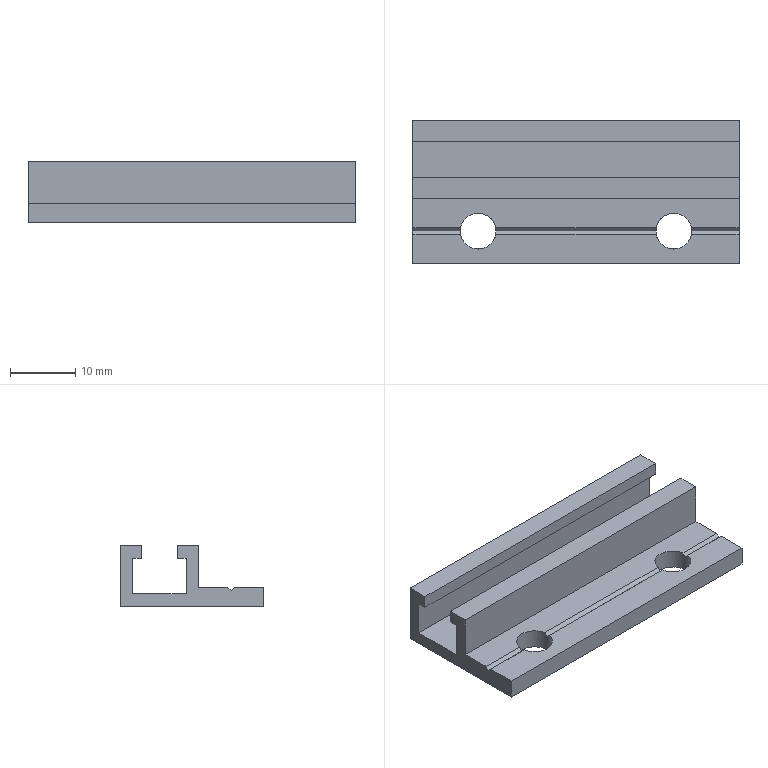Part | STEP file | SENCF5-50 | 1 solid | 27 faces | box 50 x 22 x 9.5 mm | volume 4243 mm3 | plane 23 | cylinder 4 | commonest cylinder face diameters 5.5 x4
STEP:
#1=CARTESIAN_POINT('',(42.704,-0.5,3.));
#2=VERTEX_POINT('',#1);
#3=CARTESIAN_POINT('',(42.75,0.,2.5));
#4=VERTEX_POINT('',#3);
#5=CARTESIAN_POINT('',(42.704,-0.5,3.));
#6=CARTESIAN_POINT('',(42.735,-0.335,2.835));
#7=CARTESIAN_POINT('',(42.75,-0.1678,2.668));
#8=CARTESIAN_POINT('',(42.75,0.,2.5));
#9=(BOUNDED_CURVE()B_SPLINE_CURVE(3,(#5,#6,#7,#8),.UNSPECIFIED.,.F.,.F.)B_SPLINE_CURVE_WITH_KNOTS((4,4),(4.53,4.712),.UNSPECIFIED.)CURVE()GEOMETRIC_REPRESENTATION_ITEM()RATIONAL_B_SPLINE_CURVE((1.,0.9972,0.9972,1.))REPRESENTATION_ITEM(''));
#10=EDGE_CURVE('',#2,#4,#9,.T.);
#11=ORIENTED_EDGE('',*,*,#10,.T.);
#12=CARTESIAN_POINT('',(42.75,0.,0.));
#13=VERTEX_POINT('',#12);
#14=CARTESIAN_POINT('',(42.75,0.,9.5));
#15=DIRECTION('',(0.,0.,-1.));
#16=VECTOR('',#15,1000.);
#17=LINE('',#14,#16);
#18=EDGE_CURVE('',#4,#13,#17,.T.);
#19=ORIENTED_EDGE('',*,*,#18,.T.);
#20=CARTESIAN_POINT('',(37.25,0.,0.));
#21=VERTEX_POINT('',#20);
#22=CARTESIAN_POINT('',(40.,0.,0.));
#23=DIRECTION('',(0.,0.,1.));
#24=DIRECTION('',(1.,0.,0.));
#25=AXIS2_PLACEMENT_3D('',#22,#23,#24);
#26=CIRCLE('',#25,2.75);
#27=EDGE_CURVE('',#21,#13,#26,.T.);
#28=ORIENTED_EDGE('',*,*,#27,.F.);
#29=CARTESIAN_POINT('',(37.25,0.,2.5));
#30=VERTEX_POINT('',#29);
#31=CARTESIAN_POINT('',(37.25,0.,9.5));
#32=DIRECTION('',(0.,0.,-1.));
#33=VECTOR('',#32,1000.);
#34=LINE('',#31,#33);
#35=EDGE_CURVE('',#30,#21,#34,.T.);
#36=ORIENTED_EDGE('',*,*,#35,.F.);
#37=CARTESIAN_POINT('',(37.296,-0.5,3.));
#38=VERTEX_POINT('',#37);
#39=CARTESIAN_POINT('',(37.25,0.,2.5));
#40=CARTESIAN_POINT('',(37.25,-0.1678,2.668));
#41=CARTESIAN_POINT('',(37.265,-0.335,2.835));
#42=CARTESIAN_POINT('',(37.296,-0.5,3.));
#43=(BOUNDED_CURVE()B_SPLINE_CURVE(3,(#39,#40,#41,#42),.UNSPECIFIED.,.F.,.F.)B_SPLINE_CURVE_WITH_KNOTS((4,4),(1.571,1.754),.UNSPECIFIED.)CURVE()GEOMETRIC_REPRESENTATION_ITEM()RATIONAL_B_SPLINE_CURVE((1.,0.9972,0.9972,1.))REPRESENTATION_ITEM(''));
#44=EDGE_CURVE('',#30,#38,#43,.T.);
#45=ORIENTED_EDGE('',*,*,#44,.T.);
#46=CARTESIAN_POINT('',(40.,0.,3.));
#47=DIRECTION('',(0.,0.,1.));
#48=DIRECTION('',(0.,1.,0.));
#49=AXIS2_PLACEMENT_3D('',#46,#47,#48);
#50=CIRCLE('',#49,2.75);
#51=EDGE_CURVE('',#38,#2,#50,.T.);
#52=ORIENTED_EDGE('',*,*,#51,.T.);
#53=EDGE_LOOP('',(#11,#19,#28,#36,#45,#52));
#54=FACE_OUTER_BOUND('',#53,.T.);
#55=CARTESIAN_POINT('',(40.,0.,9.5));
#56=DIRECTION('',(0.,0.,-1.));
#57=DIRECTION('',(-1.,0.,0.));
#58=AXIS2_PLACEMENT_3D('',#55,#56,#57);
#59=CYLINDRICAL_SURFACE('',#58,2.75);
#60=ADVANCED_FACE('',(#54),#59,.F.);
#61=CARTESIAN_POINT('',(12.704,-0.5,3.));
#62=VERTEX_POINT('',#61);
#63=CARTESIAN_POINT('',(12.75,0.,2.5));
#64=VERTEX_POINT('',#63);
#65=CARTESIAN_POINT('',(12.704,-0.5,3.));
#66=CARTESIAN_POINT('',(12.735,-0.335,2.835));
#67=CARTESIAN_POINT('',(12.75,-0.1678,2.668));
#68=CARTESIAN_POINT('',(12.75,0.,2.5));
#69=(BOUNDED_CURVE()B_SPLINE_CURVE(3,(#65,#66,#67,#68),.UNSPECIFIED.,.F.,.F.)B_SPLINE_CURVE_WITH_KNOTS((4,4),(4.53,4.712),.UNSPECIFIED.)CURVE()GEOMETRIC_REPRESENTATION_ITEM()RATIONAL_B_SPLINE_CURVE((1.,0.9972,0.9972,1.))REPRESENTATION_ITEM(''));
#70=EDGE_CURVE('',#62,#64,#69,.T.);
#71=ORIENTED_EDGE('',*,*,#70,.T.);
#72=CARTESIAN_POINT('',(12.75,0.,0.));
#73=VERTEX_POINT('',#72);
#74=CARTESIAN_POINT('',(12.75,0.,9.5));
#75=DIRECTION('',(0.,0.,-1.));
#76=VECTOR('',#75,1000.);
#77=LINE('',#74,#76);
#78=EDGE_CURVE('',#64,#73,#77,.T.);
#79=ORIENTED_EDGE('',*,*,#78,.T.);
#80=CARTESIAN_POINT('',(7.25,0.,0.));
#81=VERTEX_POINT('',#80);
#82=CARTESIAN_POINT('',(10.,0.,0.));
#83=DIRECTION('',(0.,0.,1.));
#84=DIRECTION('',(1.,0.,0.));
#85=AXIS2_PLACEMENT_3D('',#82,#83,#84);
#86=CIRCLE('',#85,2.75);
#87=EDGE_CURVE('',#81,#73,#86,.T.);
#88=ORIENTED_EDGE('',*,*,#87,.F.);
#89=CARTESIAN_POINT('',(7.25,0.,2.5));
#90=VERTEX_POINT('',#89);
#91=CARTESIAN_POINT('',(7.25,0.,9.5));
#92=DIRECTION('',(0.,0.,-1.));
#93=VECTOR('',#92,1000.);
#94=LINE('',#91,#93);
#95=EDGE_CURVE('',#90,#81,#94,.T.);
#96=ORIENTED_EDGE('',*,*,#95,.F.);
#97=CARTESIAN_POINT('',(7.296,-0.5,3.));
#98=VERTEX_POINT('',#97);
#99=CARTESIAN_POINT('',(7.25,0.,2.5));
#100=CARTESIAN_POINT('',(7.25,-0.1678,2.668));
#101=CARTESIAN_POINT('',(7.265,-0.335,2.835));
#102=CARTESIAN_POINT('',(7.296,-0.5,3.));
#103=(BOUNDED_CURVE()B_SPLINE_CURVE(3,(#99,#100,#101,#102),.UNSPECIFIED.,.F.,.F.)B_SPLINE_CURVE_WITH_KNOTS((4,4),(1.571,1.754),.UNSPECIFIED.)CURVE()GEOMETRIC_REPRESENTATION_ITEM()RATIONAL_B_SPLINE_CURVE((1.,0.9972,0.9972,1.))REPRESENTATION_ITEM(''));
#104=EDGE_CURVE('',#90,#98,#103,.T.);
#105=ORIENTED_EDGE('',*,*,#104,.T.);
#106=CARTESIAN_POINT('',(10.,0.,3.));
#107=DIRECTION('',(0.,0.,1.));
#108=DIRECTION('',(0.,1.,0.));
#109=AXIS2_PLACEMENT_3D('',#106,#107,#108);
#110=CIRCLE('',#109,2.75);
#111=EDGE_CURVE('',#98,#62,#110,.T.);
#112=ORIENTED_EDGE('',*,*,#111,.T.);
#113=EDGE_LOOP('',(#71,#79,#88,#96,#105,#112));
#114=FACE_OUTER_BOUND('',#113,.T.);
#115=CARTESIAN_POINT('',(10.,0.,9.5));
#116=DIRECTION('',(0.,0.,-1.));
#117=DIRECTION('',(-1.,0.,0.));
#118=AXIS2_PLACEMENT_3D('',#115,#116,#117);
#119=CYLINDRICAL_SURFACE('',#118,2.75);
#120=ADVANCED_FACE('',(#114),#119,.F.);
#121=CARTESIAN_POINT('',(0.,-5.,0.));
#122=VERTEX_POINT('',#121);
#123=CARTESIAN_POINT('',(0.,17.,0.));
#124=VERTEX_POINT('',#123);
#125=CARTESIAN_POINT('',(0.,-5.,0.));
#126=DIRECTION('',(0.,1.,0.));
#127=VECTOR('',#126,1000.);
#128=LINE('',#125,#127);
#129=EDGE_CURVE('',#122,#124,#128,.T.);
#130=ORIENTED_EDGE('',*,*,#129,.T.);
#131=CARTESIAN_POINT('',(50.,17.,0.));
#132=VERTEX_POINT('',#131);
#133=CARTESIAN_POINT('',(50.,17.,0.));
#134=DIRECTION('',(-1.,0.,0.));
#135=VECTOR('',#134,1000.);
#136=LINE('',#133,#135);
#137=EDGE_CURVE('',#132,#124,#136,.T.);
#138=ORIENTED_EDGE('',*,*,#137,.F.);
#139=CARTESIAN_POINT('',(50.,-5.,0.));
#140=VERTEX_POINT('',#139);
#141=CARTESIAN_POINT('',(50.,-5.,0.));
#142=DIRECTION('',(0.,1.,0.));
#143=VECTOR('',#142,1000.);
#144=LINE('',#141,#143);
#145=EDGE_CURVE('',#140,#132,#144,.T.);
#146=ORIENTED_EDGE('',*,*,#145,.F.);
#147=CARTESIAN_POINT('',(50.,-5.,0.));
#148=DIRECTION('',(-1.,0.,0.));
#149=VECTOR('',#148,1000.);
#150=LINE('',#147,#149);
#151=EDGE_CURVE('',#140,#122,#150,.T.);
#152=ORIENTED_EDGE('',*,*,#151,.T.);
#153=EDGE_LOOP('',(#130,#138,#146,#152));
#154=FACE_OUTER_BOUND('',#153,.T.);
#155=ORIENTED_EDGE('',*,*,#87,.T.);
#156=CARTESIAN_POINT('',(10.,0.,0.));
#157=DIRECTION('',(0.,0.,1.));
#158=DIRECTION('',(1.,0.,0.));
#159=AXIS2_PLACEMENT_3D('',#156,#157,#158);
#160=CIRCLE('',#159,2.75);
#161=EDGE_CURVE('',#73,#81,#160,.T.);
#162=ORIENTED_EDGE('',*,*,#161,.T.);
#163=EDGE_LOOP('',(#155,#162));
#164=FACE_BOUND('',#163,.T.);
#165=ORIENTED_EDGE('',*,*,#27,.T.);
#166=CARTESIAN_POINT('',(40.,0.,0.));
#167=DIRECTION('',(0.,0.,1.));
#168=DIRECTION('',(1.,0.,0.));
#169=AXIS2_PLACEMENT_3D('',#166,#167,#168);
#170=CIRCLE('',#169,2.75);
#171=EDGE_CURVE('',#13,#21,#170,.T.);
#172=ORIENTED_EDGE('',*,*,#171,.T.);
#173=EDGE_LOOP('',(#165,#172));
#174=FACE_BOUND('',#173,.T.);
#175=CARTESIAN_POINT('',(50.,-5.,0.));
#176=DIRECTION('',(0.,0.,1.));
#177=DIRECTION('',(0.,-1.,0.));
#178=AXIS2_PLACEMENT_3D('',#175,#176,#177);
#179=PLANE('',#178);
#180=ADVANCED_FACE('',(#154,#164,#174),#179,.F.);
#181=CARTESIAN_POINT('',(42.704,0.5,3.));
#182=VERTEX_POINT('',#181);
#183=CARTESIAN_POINT('',(37.296,0.5,3.));
#184=VERTEX_POINT('',#183);
#185=CARTESIAN_POINT('',(40.,0.,3.));
#186=DIRECTION('',(0.,0.,1.));
#187=DIRECTION('',(0.,1.,0.));
#188=AXIS2_PLACEMENT_3D('',#185,#186,#187);
#189=CIRCLE('',#188,2.75);
#190=EDGE_CURVE('',#182,#184,#189,.T.);
#191=ORIENTED_EDGE('',*,*,#190,.F.);
#192=CARTESIAN_POINT('',(50.,0.5,3.));
#193=VERTEX_POINT('',#192);
#194=CARTESIAN_POINT('',(50.,0.5,3.));
#195=DIRECTION('',(-1.,0.,0.));
#196=VECTOR('',#195,1000.);
#197=LINE('',#194,#196);
#198=EDGE_CURVE('',#193,#182,#197,.T.);
#199=ORIENTED_EDGE('',*,*,#198,.F.);
#200=CARTESIAN_POINT('',(50.,5.,3.));
#201=VERTEX_POINT('',#200);
#202=CARTESIAN_POINT('',(50.,5.,3.));
#203=DIRECTION('',(0.,-1.,0.));
#204=VECTOR('',#203,1000.);
#205=LINE('',#202,#204);
#206=EDGE_CURVE('',#201,#193,#205,.T.);
#207=ORIENTED_EDGE('',*,*,#206,.F.);
#208=CARTESIAN_POINT('',(0.,5.,3.));
#209=VERTEX_POINT('',#208);
#210=CARTESIAN_POINT('',(50.,5.,3.));
#211=DIRECTION('',(-1.,0.,0.));
#212=VECTOR('',#211,1000.);
#213=LINE('',#210,#212);
#214=EDGE_CURVE('',#201,#209,#213,.T.);
#215=ORIENTED_EDGE('',*,*,#214,.T.);
#216=CARTESIAN_POINT('',(0.,0.5,3.));
#217=VERTEX_POINT('',#216);
#218=CARTESIAN_POINT('',(0.,5.,3.));
#219=DIRECTION('',(0.,-1.,0.));
#220=VECTOR('',#219,1000.);
#221=LINE('',#218,#220);
#222=EDGE_CURVE('',#209,#217,#221,.T.);
#223=ORIENTED_EDGE('',*,*,#222,.T.);
#224=CARTESIAN_POINT('',(7.296,0.5,3.));
#225=VERTEX_POINT('',#224);
#226=CARTESIAN_POINT('',(50.,0.5,3.));
#227=DIRECTION('',(-1.,0.,0.));
#228=VECTOR('',#227,1000.);
#229=LINE('',#226,#228);
#230=EDGE_CURVE('',#225,#217,#229,.T.);
#231=ORIENTED_EDGE('',*,*,#230,.F.);
#232=CARTESIAN_POINT('',(12.704,0.5,3.));
#233=VERTEX_POINT('',#232);
#234=CARTESIAN_POINT('',(10.,0.,3.));
#235=DIRECTION('',(0.,0.,1.));
#236=DIRECTION('',(0.,1.,0.));
#237=AXIS2_PLACEMENT_3D('',#234,#235,#236);
#238=CIRCLE('',#237,2.75);
#239=EDGE_CURVE('',#233,#225,#238,.T.);
#240=ORIENTED_EDGE('',*,*,#239,.F.);
#241=CARTESIAN_POINT('',(50.,0.5,3.));
#242=DIRECTION('',(-1.,0.,0.));
#243=VECTOR('',#242,1000.);
#244=LINE('',#241,#243);
#245=EDGE_CURVE('',#184,#233,#244,.T.);
#246=ORIENTED_EDGE('',*,*,#245,.F.);
#247=EDGE_LOOP('',(#191,#199,#207,#215,#223,#231,#240,#246));
#248=FACE_OUTER_BOUND('',#247,.T.);
#249=CARTESIAN_POINT('',(50.,5.,3.));
#250=DIRECTION('',(0.,0.,-1.));
#251=DIRECTION('',(0.,1.,0.));
#252=AXIS2_PLACEMENT_3D('',#249,#250,#251);
#253=PLANE('',#252);
#254=ADVANCED_FACE('',(#248),#253,.F.);
#255=CARTESIAN_POINT('',(42.75,0.,2.5));
#256=CARTESIAN_POINT('',(42.75,0.1678,2.668));
#257=CARTESIAN_POINT('',(42.735,0.335,2.835));
#258=CARTESIAN_POINT('',(42.704,0.5,3.));
#259=(BOUNDED_CURVE()B_SPLINE_CURVE(3,(#255,#256,#257,#258),.UNSPECIFIED.,.F.,.F.)B_SPLINE_CURVE_WITH_KNOTS((4,4),(1.571,1.754),.UNSPECIFIED.)CURVE()GEOMETRIC_REPRESENTATION_ITEM()RATIONAL_B_SPLINE_CURVE((1.,0.9972,0.9972,1.))REPRESENTATION_ITEM(''));
#260=EDGE_CURVE('',#4,#182,#259,.T.);
#261=ORIENTED_EDGE('',*,*,#260,.F.);
#262=CARTESIAN_POINT('',(50.,0.,2.5));
#263=VERTEX_POINT('',#262);
#264=CARTESIAN_POINT('',(50.,0.,2.5));
#265=DIRECTION('',(-1.,0.,0.));
#266=VECTOR('',#265,1000.);
#267=LINE('',#264,#266);
#268=EDGE_CURVE('',#263,#4,#267,.T.);
#269=ORIENTED_EDGE('',*,*,#268,.F.);
#270=CARTESIAN_POINT('',(50.,0.5,3.));
#271=DIRECTION('',(0.,-0.7071,-0.7071));
#272=VECTOR('',#271,1000.);
#273=LINE('',#270,#272);
#274=EDGE_CURVE('',#193,#263,#273,.T.);
#275=ORIENTED_EDGE('',*,*,#274,.F.);
#276=ORIENTED_EDGE('',*,*,#198,.T.);
#277=EDGE_LOOP('',(#261,#269,#275,#276));
#278=FACE_OUTER_BOUND('',#277,.T.);
#279=CARTESIAN_POINT('',(50.,0.5,3.));
#280=DIRECTION('',(0.,0.7071,-0.7071));
#281=DIRECTION('',(0.,0.7071,0.7071));
#282=AXIS2_PLACEMENT_3D('',#279,#280,#281);
#283=PLANE('',#282);
#284=ADVANCED_FACE('',(#278),#283,.F.);
#285=CARTESIAN_POINT('',(37.296,0.5,3.));
#286=CARTESIAN_POINT('',(37.265,0.335,2.835));
#287=CARTESIAN_POINT('',(37.25,0.1678,2.668));
#288=CARTESIAN_POINT('',(37.25,0.,2.5));
#289=(BOUNDED_CURVE()B_SPLINE_CURVE(3,(#285,#286,#287,#288),.UNSPECIFIED.,.F.,.F.)B_SPLINE_CURVE_WITH_KNOTS((4,4),(4.53,4.712),.UNSPECIFIED.)CURVE()GEOMETRIC_REPRESENTATION_ITEM()RATIONAL_B_SPLINE_CURVE((1.,0.9972,0.9972,1.))REPRESENTATION_ITEM(''));
#290=EDGE_CURVE('',#184,#30,#289,.T.);
#291=ORIENTED_EDGE('',*,*,#290,.F.);
#292=ORIENTED_EDGE('',*,*,#245,.T.);
#293=CARTESIAN_POINT('',(12.75,0.,2.5));
#294=CARTESIAN_POINT('',(12.75,0.1678,2.668));
#295=CARTESIAN_POINT('',(12.735,0.335,2.835));
#296=CARTESIAN_POINT('',(12.704,0.5,3.));
#297=(BOUNDED_CURVE()B_SPLINE_CURVE(3,(#293,#294,#295,#296),.UNSPECIFIED.,.F.,.F.)B_SPLINE_CURVE_WITH_KNOTS((4,4),(1.571,1.754),.UNSPECIFIED.)CURVE()GEOMETRIC_REPRESENTATION_ITEM()RATIONAL_B_SPLINE_CURVE((1.,0.9972,0.9972,1.))REPRESENTATION_ITEM(''));
#298=EDGE_CURVE('',#64,#233,#297,.T.);
#299=ORIENTED_EDGE('',*,*,#298,.F.);
#300=CARTESIAN_POINT('',(50.,0.,2.5));
#301=DIRECTION('',(-1.,0.,0.));
#302=VECTOR('',#301,1000.);
#303=LINE('',#300,#302);
#304=EDGE_CURVE('',#30,#64,#303,.T.);
#305=ORIENTED_EDGE('',*,*,#304,.F.);
#306=EDGE_LOOP('',(#291,#292,#299,#305));
#307=FACE_OUTER_BOUND('',#306,.T.);
#308=CARTESIAN_POINT('',(50.,0.5,3.));
#309=DIRECTION('',(0.,0.7071,-0.7071));
#310=DIRECTION('',(0.,0.7071,0.7071));
#311=AXIS2_PLACEMENT_3D('',#308,#309,#310);
#312=PLANE('',#311);
#313=ADVANCED_FACE('',(#307),#312,.F.);
#314=ORIENTED_EDGE('',*,*,#44,.F.);
#315=ORIENTED_EDGE('',*,*,#304,.T.);
#316=ORIENTED_EDGE('',*,*,#70,.F.);
#317=CARTESIAN_POINT('',(50.,-0.5,3.));
#318=DIRECTION('',(-1.,0.,0.));
#319=VECTOR('',#318,1000.);
#320=LINE('',#317,#319);
#321=EDGE_CURVE('',#38,#62,#320,.T.);
#322=ORIENTED_EDGE('',*,*,#321,.F.);
#323=EDGE_LOOP('',(#314,#315,#316,#322));
#324=FACE_OUTER_BOUND('',#323,.T.);
#325=CARTESIAN_POINT('',(50.,0.,2.5));
#326=DIRECTION('',(0.,-0.7071,-0.7071));
#327=DIRECTION('',(0.,0.7071,-0.7071));
#328=AXIS2_PLACEMENT_3D('',#325,#326,#327);
#329=PLANE('',#328);
#330=ADVANCED_FACE('',(#324),#329,.F.);
#331=ORIENTED_EDGE('',*,*,#10,.F.);
#332=CARTESIAN_POINT('',(50.,-0.5,3.));
#333=VERTEX_POINT('',#332);
#334=CARTESIAN_POINT('',(50.,-0.5,3.));
#335=DIRECTION('',(-1.,0.,0.));
#336=VECTOR('',#335,1000.);
#337=LINE('',#334,#336);
#338=EDGE_CURVE('',#333,#2,#337,.T.);
#339=ORIENTED_EDGE('',*,*,#338,.F.);
#340=CARTESIAN_POINT('',(50.,0.,2.5));
#341=DIRECTION('',(0.,-0.7071,0.7071));
#342=VECTOR('',#341,1000.);
#343=LINE('',#340,#342);
#344=EDGE_CURVE('',#263,#333,#343,.T.);
#345=ORIENTED_EDGE('',*,*,#344,.F.);
#346=ORIENTED_EDGE('',*,*,#268,.T.);
#347=EDGE_LOOP('',(#331,#339,#345,#346));
#348=FACE_OUTER_BOUND('',#347,.T.);
#349=CARTESIAN_POINT('',(50.,0.,2.5));
#350=DIRECTION('',(0.,-0.7071,-0.7071));
#351=DIRECTION('',(0.,0.7071,-0.7071));
#352=AXIS2_PLACEMENT_3D('',#349,#350,#351);
#353=PLANE('',#352);
#354=ADVANCED_FACE('',(#348),#353,.F.);
#355=ORIENTED_EDGE('',*,*,#51,.F.);
#356=ORIENTED_EDGE('',*,*,#321,.T.);
#357=ORIENTED_EDGE('',*,*,#111,.F.);
#358=CARTESIAN_POINT('',(0.,-0.5,3.));
#359=VERTEX_POINT('',#358);
#360=CARTESIAN_POINT('',(50.,-0.5,3.));
#361=DIRECTION('',(-1.,0.,0.));
#362=VECTOR('',#361,1000.);
#363=LINE('',#360,#362);
#364=EDGE_CURVE('',#98,#359,#363,.T.);
#365=ORIENTED_EDGE('',*,*,#364,.T.);
#366=CARTESIAN_POINT('',(0.,-5.,3.));
#367=VERTEX_POINT('',#366);
#368=CARTESIAN_POINT('',(0.,-0.5,3.));
#369=DIRECTION('',(0.,-1.,0.));
#370=VECTOR('',#369,1000.);
#371=LINE('',#368,#370);
#372=EDGE_CURVE('',#359,#367,#371,.T.);
#373=ORIENTED_EDGE('',*,*,#372,.T.);
#374=CARTESIAN_POINT('',(50.,-5.,3.));
#375=VERTEX_POINT('',#374);
#376=CARTESIAN_POINT('',(50.,-5.,3.));
#377=DIRECTION('',(-1.,0.,0.));
#378=VECTOR('',#377,1000.);
#379=LINE('',#376,#378);
#380=EDGE_CURVE('',#375,#367,#379,.T.);
#381=ORIENTED_EDGE('',*,*,#380,.F.);
#382=CARTESIAN_POINT('',(50.,-0.5,3.));
#383=DIRECTION('',(0.,-1.,0.));
#384=VECTOR('',#383,1000.);
#385=LINE('',#382,#384);
#386=EDGE_CURVE('',#333,#375,#385,.T.);
#387=ORIENTED_EDGE('',*,*,#386,.F.);
#388=ORIENTED_EDGE('',*,*,#338,.T.);
#389=EDGE_LOOP('',(#355,#356,#357,#365,#373,#381,#387,#388));
#390=FACE_OUTER_BOUND('',#389,.T.);
#391=CARTESIAN_POINT('',(50.,-0.5,3.));
#392=DIRECTION('',(0.,0.,-1.));
#393=DIRECTION('',(0.,1.,0.));
#394=AXIS2_PLACEMENT_3D('',#391,#392,#393);
#395=PLANE('',#394);
#396=ADVANCED_FACE('',(#390),#395,.F.);
#397=CARTESIAN_POINT('',(7.296,0.5,3.));
#398=CARTESIAN_POINT('',(7.265,0.335,2.835));
#399=CARTESIAN_POINT('',(7.25,0.1678,2.668));
#400=CARTESIAN_POINT('',(7.25,0.,2.5));
#401=(BOUNDED_CURVE()B_SPLINE_CURVE(3,(#397,#398,#399,#400),.UNSPECIFIED.,.F.,.F.)B_SPLINE_CURVE_WITH_KNOTS((4,4),(4.53,4.712),.UNSPECIFIED.)CURVE()GEOMETRIC_REPRESENTATION_ITEM()RATIONAL_B_SPLINE_CURVE((1.,0.9972,0.9972,1.))REPRESENTATION_ITEM(''));
#402=EDGE_CURVE('',#225,#90,#401,.T.);
#403=ORIENTED_EDGE('',*,*,#402,.F.);
#404=ORIENTED_EDGE('',*,*,#230,.T.);
#405=CARTESIAN_POINT('',(0.,0.,2.5));
#406=VERTEX_POINT('',#405);
#407=CARTESIAN_POINT('',(0.,0.5,3.));
#408=DIRECTION('',(0.,-0.7071,-0.7071));
#409=VECTOR('',#408,1000.);
#410=LINE('',#407,#409);
#411=EDGE_CURVE('',#217,#406,#410,.T.);
#412=ORIENTED_EDGE('',*,*,#411,.T.);
#413=CARTESIAN_POINT('',(50.,0.,2.5));
#414=DIRECTION('',(-1.,0.,0.));
#415=VECTOR('',#414,1000.);
#416=LINE('',#413,#415);
#417=EDGE_CURVE('',#90,#406,#416,.T.);
#418=ORIENTED_EDGE('',*,*,#417,.F.);
#419=EDGE_LOOP('',(#403,#404,#412,#418));
#420=FACE_OUTER_BOUND('',#419,.T.);
#421=CARTESIAN_POINT('',(50.,0.5,3.));
#422=DIRECTION('',(0.,0.7071,-0.7071));
#423=DIRECTION('',(0.,0.7071,0.7071));
#424=AXIS2_PLACEMENT_3D('',#421,#422,#423);
#425=PLANE('',#424);
#426=ADVANCED_FACE('',(#420),#425,.F.);
#427=ORIENTED_EDGE('',*,*,#104,.F.);
#428=ORIENTED_EDGE('',*,*,#417,.T.);
#429=CARTESIAN_POINT('',(0.,0.,2.5));
#430=DIRECTION('',(0.,-0.7071,0.7071));
#431=VECTOR('',#430,1000.);
#432=LINE('',#429,#431);
#433=EDGE_CURVE('',#406,#359,#432,.T.);
#434=ORIENTED_EDGE('',*,*,#433,.T.);
#435=ORIENTED_EDGE('',*,*,#364,.F.);
#436=EDGE_LOOP('',(#427,#428,#434,#435));
#437=FACE_OUTER_BOUND('',#436,.T.);
#438=CARTESIAN_POINT('',(50.,0.,2.5));
#439=DIRECTION('',(0.,-0.7071,-0.7071));
#440=DIRECTION('',(0.,0.7071,-0.7071));
#441=AXIS2_PLACEMENT_3D('',#438,#439,#440);
#442=PLANE('',#441);
#443=ADVANCED_FACE('',(#437),#442,.F.);
#444=CARTESIAN_POINT('',(0.,17.,9.5));
#445=VERTEX_POINT('',#444);
#446=CARTESIAN_POINT('',(0.,17.,0.));
#447=DIRECTION('',(0.,0.,1.));
#448=VECTOR('',#447,1000.);
#449=LINE('',#446,#448);
#450=EDGE_CURVE('',#124,#445,#449,.T.);
#451=ORIENTED_EDGE('',*,*,#450,.T.);
#452=CARTESIAN_POINT('',(50.,17.,9.5));
#453=VERTEX_POINT('',#452);
#454=CARTESIAN_POINT('',(50.,17.,9.5));
#455=DIRECTION('',(-1.,0.,0.));
#456=VECTOR('',#455,1000.);
#457=LINE('',#454,#456);
#458=EDGE_CURVE('',#453,#445,#457,.T.);
#459=ORIENTED_EDGE('',*,*,#458,.F.);
#460=CARTESIAN_POINT('',(50.,17.,0.));
#461=DIRECTION('',(0.,0.,1.));
#462=VECTOR('',#461,1000.);
#463=LINE('',#460,#462);
#464=EDGE_CURVE('',#132,#453,#463,.T.);
#465=ORIENTED_EDGE('',*,*,#464,.F.);
#466=ORIENTED_EDGE('',*,*,#137,.T.);
#467=EDGE_LOOP('',(#451,#459,#465,#466));
#468=FACE_OUTER_BOUND('',#467,.T.);
#469=CARTESIAN_POINT('',(50.,17.,0.));
#470=DIRECTION('',(0.,-1.,0.));
#471=DIRECTION('',(0.,0.,-1.));
#472=AXIS2_PLACEMENT_3D('',#469,#470,#471);
#473=PLANE('',#472);
#474=ADVANCED_FACE('',(#468),#473,.F.);
#475=CARTESIAN_POINT('',(0.,13.75,9.5));
#476=VERTEX_POINT('',#475);
#477=CARTESIAN_POINT('',(0.,17.,9.5));
#478=DIRECTION('',(0.,-1.,0.));
#479=VECTOR('',#478,1000.);
#480=LINE('',#477,#479);
#481=EDGE_CURVE('',#445,#476,#480,.T.);
#482=ORIENTED_EDGE('',*,*,#481,.T.);
#483=CARTESIAN_POINT('',(50.,13.75,9.5));
#484=VERTEX_POINT('',#483);
#485=CARTESIAN_POINT('',(50.,13.75,9.5));
#486=DIRECTION('',(-1.,0.,0.));
#487=VECTOR('',#486,1000.);
#488=LINE('',#485,#487);
#489=EDGE_CURVE('',#484,#476,#488,.T.);
#490=ORIENTED_EDGE('',*,*,#489,.F.);
#491=CARTESIAN_POINT('',(50.,17.,9.5));
#492=DIRECTION('',(0.,-1.,0.));
#493=VECTOR('',#492,1000.);
#494=LINE('',#491,#493);
#495=EDGE_CURVE('',#453,#484,#494,.T.);
#496=ORIENTED_EDGE('',*,*,#495,.F.);
#497=ORIENTED_EDGE('',*,*,#458,.T.);
#498=EDGE_LOOP('',(#482,#490,#496,#497));
#499=FACE_OUTER_BOUND('',#498,.T.);
#500=CARTESIAN_POINT('',(50.,17.,9.5));
#501=DIRECTION('',(0.,0.,-1.));
#502=DIRECTION('',(0.,1.,0.));
#503=AXIS2_PLACEMENT_3D('',#500,#501,#502);
#504=PLANE('',#503);
#505=ADVANCED_FACE('',(#499),#504,.F.);
#506=CARTESIAN_POINT('',(0.,13.75,7.5));
#507=VERTEX_POINT('',#506);
#508=CARTESIAN_POINT('',(0.,13.75,9.5));
#509=DIRECTION('',(0.,0.,-1.));
#510=VECTOR('',#509,1000.);
#511=LINE('',#508,#510);
#512=EDGE_CURVE('',#476,#507,#511,.T.);
#513=ORIENTED_EDGE('',*,*,#512,.T.);
#514=CARTESIAN_POINT('',(50.,13.75,7.5));
#515=VERTEX_POINT('',#514);
#516=CARTESIAN_POINT('',(50.,13.75,7.5));
#517=DIRECTION('',(-1.,0.,0.));
#518=VECTOR('',#517,1000.);
#519=LINE('',#516,#518);
#520=EDGE_CURVE('',#515,#507,#519,.T.);
#521=ORIENTED_EDGE('',*,*,#520,.F.);
#522=CARTESIAN_POINT('',(50.,13.75,9.5));
#523=DIRECTION('',(0.,0.,-1.));
#524=VECTOR('',#523,1000.);
#525=LINE('',#522,#524);
#526=EDGE_CURVE('',#484,#515,#525,.T.);
#527=ORIENTED_EDGE('',*,*,#526,.F.);
#528=ORIENTED_EDGE('',*,*,#489,.T.);
#529=EDGE_LOOP('',(#513,#521,#527,#528));
#530=FACE_OUTER_BOUND('',#529,.T.);
#531=CARTESIAN_POINT('',(50.,13.75,9.5));
#532=DIRECTION('',(0.,1.,0.));
#533=DIRECTION('',(0.,0.,1.));
#534=AXIS2_PLACEMENT_3D('',#531,#532,#533);
#535=PLANE('',#534);
#536=ADVANCED_FACE('',(#530),#535,.F.);
#537=CARTESIAN_POINT('',(0.,15.1,7.5));
#538=VERTEX_POINT('',#537);
#539=CARTESIAN_POINT('',(0.,13.75,7.5));
#540=DIRECTION('',(0.,1.,0.));
#541=VECTOR('',#540,1000.);
#542=LINE('',#539,#541);
#543=EDGE_CURVE('',#507,#538,#542,.T.);
#544=ORIENTED_EDGE('',*,*,#543,.T.);
#545=CARTESIAN_POINT('',(50.,15.1,7.5));
#546=VERTEX_POINT('',#545);
#547=CARTESIAN_POINT('',(50.,15.1,7.5));
#548=DIRECTION('',(-1.,0.,0.));
#549=VECTOR('',#548,1000.);
#550=LINE('',#547,#549);
#551=EDGE_CURVE('',#546,#538,#550,.T.);
#552=ORIENTED_EDGE('',*,*,#551,.F.);
#553=CARTESIAN_POINT('',(50.,13.75,7.5));
#554=DIRECTION('',(0.,1.,0.));
#555=VECTOR('',#554,1000.);
#556=LINE('',#553,#555);
#557=EDGE_CURVE('',#515,#546,#556,.T.);
#558=ORIENTED_EDGE('',*,*,#557,.F.);
#559=ORIENTED_EDGE('',*,*,#520,.T.);
#560=EDGE_LOOP('',(#544,#552,#558,#559));
#561=FACE_OUTER_BOUND('',#560,.T.);
#562=CARTESIAN_POINT('',(50.,13.75,7.5));
#563=DIRECTION('',(0.,0.,1.));
#564=DIRECTION('',(1.,0.,0.));
#565=AXIS2_PLACEMENT_3D('',#562,#563,#564);
#566=PLANE('',#565);
#567=ADVANCED_FACE('',(#561),#566,.F.);
#568=CARTESIAN_POINT('',(0.,15.1,2.));
#569=VERTEX_POINT('',#568);
#570=CARTESIAN_POINT('',(0.,15.1,7.5));
#571=DIRECTION('',(0.,0.,-1.));
#572=VECTOR('',#571,1000.);
#573=LINE('',#570,#572);
#574=EDGE_CURVE('',#538,#569,#573,.T.);
#575=ORIENTED_EDGE('',*,*,#574,.T.);
#576=CARTESIAN_POINT('',(50.,15.1,2.));
#577=VERTEX_POINT('',#576);
#578=CARTESIAN_POINT('',(50.,15.1,2.));
#579=DIRECTION('',(-1.,0.,0.));
#580=VECTOR('',#579,1000.);
#581=LINE('',#578,#580);
#582=EDGE_CURVE('',#577,#569,#581,.T.);
#583=ORIENTED_EDGE('',*,*,#582,.F.);
#584=CARTESIAN_POINT('',(50.,15.1,7.5));
#585=DIRECTION('',(0.,0.,-1.));
#586=VECTOR('',#585,1000.);
#587=LINE('',#584,#586);
#588=EDGE_CURVE('',#546,#577,#587,.T.);
#589=ORIENTED_EDGE('',*,*,#588,.F.);
#590=ORIENTED_EDGE('',*,*,#551,.T.);
#591=EDGE_LOOP('',(#575,#583,#589,#590));
#592=FACE_OUTER_BOUND('',#591,.T.);
#593=CARTESIAN_POINT('',(50.,15.1,7.5));
#594=DIRECTION('',(0.,1.,0.));
#595=DIRECTION('',(0.,0.,1.));
#596=AXIS2_PLACEMENT_3D('',#593,#594,#595);
#597=PLANE('',#596);
#598=ADVANCED_FACE('',(#592),#597,.F.);
#599=CARTESIAN_POINT('',(0.,6.9,2.));
#600=VERTEX_POINT('',#599);
#601=CARTESIAN_POINT('',(0.,15.1,2.));
#602=DIRECTION('',(0.,-1.,0.));
#603=VECTOR('',#602,1000.);
#604=LINE('',#601,#603);
#605=EDGE_CURVE('',#569,#600,#604,.T.);
#606=ORIENTED_EDGE('',*,*,#605,.T.);
#607=CARTESIAN_POINT('',(50.,6.9,2.));
#608=VERTEX_POINT('',#607);
#609=CARTESIAN_POINT('',(50.,6.9,2.));
#610=DIRECTION('',(-1.,0.,0.));
#611=VECTOR('',#610,1000.);
#612=LINE('',#609,#611);
#613=EDGE_CURVE('',#608,#600,#612,.T.);
#614=ORIENTED_EDGE('',*,*,#613,.F.);
#615=CARTESIAN_POINT('',(50.,15.1,2.));
#616=DIRECTION('',(0.,-1.,0.));
#617=VECTOR('',#616,1000.);
#618=LINE('',#615,#617);
#619=EDGE_CURVE('',#577,#608,#618,.T.);
#620=ORIENTED_EDGE('',*,*,#619,.F.);
#621=ORIENTED_EDGE('',*,*,#582,.T.);
#622=EDGE_LOOP('',(#606,#614,#620,#621));
#623=FACE_OUTER_BOUND('',#622,.T.);
#624=CARTESIAN_POINT('',(50.,15.1,2.));
#625=DIRECTION('',(0.,0.,-1.));
#626=DIRECTION('',(0.,1.,0.));
#627=AXIS2_PLACEMENT_3D('',#624,#625,#626);
#628=PLANE('',#627);
#629=ADVANCED_FACE('',(#623),#628,.F.);
#630=CARTESIAN_POINT('',(0.,6.9,7.5));
#631=VERTEX_POINT('',#630);
#632=CARTESIAN_POINT('',(0.,6.9,2.));
#633=DIRECTION('',(0.,0.,1.));
#634=VECTOR('',#633,1000.);
#635=LINE('',#632,#634);
#636=EDGE_CURVE('',#600,#631,#635,.T.);
#637=ORIENTED_EDGE('',*,*,#636,.T.);
#638=CARTESIAN_POINT('',(50.,6.9,7.5));
#639=VERTEX_POINT('',#638);
#640=CARTESIAN_POINT('',(50.,6.9,7.5));
#641=DIRECTION('',(-1.,0.,0.));
#642=VECTOR('',#641,1000.);
#643=LINE('',#640,#642);
#644=EDGE_CURVE('',#639,#631,#643,.T.);
#645=ORIENTED_EDGE('',*,*,#644,.F.);
#646=CARTESIAN_POINT('',(50.,6.9,2.));
#647=DIRECTION('',(0.,0.,1.));
#648=VECTOR('',#647,1000.);
#649=LINE('',#646,#648);
#650=EDGE_CURVE('',#608,#639,#649,.T.);
#651=ORIENTED_EDGE('',*,*,#650,.F.);
#652=ORIENTED_EDGE('',*,*,#613,.T.);
#653=EDGE_LOOP('',(#637,#645,#651,#652));
#654=FACE_OUTER_BOUND('',#653,.T.);
#655=CARTESIAN_POINT('',(50.,6.9,2.));
#656=DIRECTION('',(0.,-1.,0.));
#657=DIRECTION('',(0.,0.,-1.));
#658=AXIS2_PLACEMENT_3D('',#655,#656,#657);
#659=PLANE('',#658);
#660=ADVANCED_FACE('',(#654),#659,.F.);
#661=CARTESIAN_POINT('',(0.,8.25,7.5));
#662=VERTEX_POINT('',#661);
#663=CARTESIAN_POINT('',(0.,6.9,7.5));
#664=DIRECTION('',(0.,1.,0.));
#665=VECTOR('',#664,1000.);
#666=LINE('',#663,#665);
#667=EDGE_CURVE('',#631,#662,#666,.T.);
#668=ORIENTED_EDGE('',*,*,#667,.T.);
#669=CARTESIAN_POINT('',(50.,8.25,7.5));
#670=VERTEX_POINT('',#669);
#671=CARTESIAN_POINT('',(50.,8.25,7.5));
#672=DIRECTION('',(-1.,0.,0.));
#673=VECTOR('',#672,1000.);
#674=LINE('',#671,#673);
#675=EDGE_CURVE('',#670,#662,#674,.T.);
#676=ORIENTED_EDGE('',*,*,#675,.F.);
#677=CARTESIAN_POINT('',(50.,6.9,7.5));
#678=DIRECTION('',(0.,1.,0.));
#679=VECTOR('',#678,1000.);
#680=LINE('',#677,#679);
#681=EDGE_CURVE('',#639,#670,#680,.T.);
#682=ORIENTED_EDGE('',*,*,#681,.F.);
#683=ORIENTED_EDGE('',*,*,#644,.T.);
#684=EDGE_LOOP('',(#668,#676,#682,#683));
#685=FACE_OUTER_BOUND('',#684,.T.);
#686=CARTESIAN_POINT('',(50.,6.9,7.5));
#687=DIRECTION('',(0.,0.,1.));
#688=DIRECTION('',(1.,0.,0.));
#689=AXIS2_PLACEMENT_3D('',#686,#687,#688);
#690=PLANE('',#689);
#691=ADVANCED_FACE('',(#685),#690,.F.);
#692=CARTESIAN_POINT('',(0.,8.25,9.5));
#693=VERTEX_POINT('',#692);
#694=CARTESIAN_POINT('',(0.,8.25,7.5));
#695=DIRECTION('',(0.,0.,1.));
#696=VECTOR('',#695,1000.);
#697=LINE('',#694,#696);
#698=EDGE_CURVE('',#662,#693,#697,.T.);
#699=ORIENTED_EDGE('',*,*,#698,.T.);
#700=CARTESIAN_POINT('',(50.,8.25,9.5));
#701=VERTEX_POINT('',#700);
#702=CARTESIAN_POINT('',(50.,8.25,9.5));
#703=DIRECTION('',(-1.,0.,0.));
#704=VECTOR('',#703,1000.);
#705=LINE('',#702,#704);
#706=EDGE_CURVE('',#701,#693,#705,.T.);
#707=ORIENTED_EDGE('',*,*,#706,.F.);
#708=CARTESIAN_POINT('',(50.,8.25,7.5));
#709=DIRECTION('',(0.,0.,1.));
#710=VECTOR('',#709,1000.);
#711=LINE('',#708,#710);
#712=EDGE_CURVE('',#670,#701,#711,.T.);
#713=ORIENTED_EDGE('',*,*,#712,.F.);
#714=ORIENTED_EDGE('',*,*,#675,.T.);
#715=EDGE_LOOP('',(#699,#707,#713,#714));
#716=FACE_OUTER_BOUND('',#715,.T.);
#717=CARTESIAN_POINT('',(50.,8.25,7.5));
#718=DIRECTION('',(0.,-1.,0.));
#719=DIRECTION('',(0.,0.,-1.));
#720=AXIS2_PLACEMENT_3D('',#717,#718,#719);
#721=PLANE('',#720);
#722=ADVANCED_FACE('',(#716),#721,.F.);
#723=CARTESIAN_POINT('',(0.,5.,9.5));
#724=VERTEX_POINT('',#723);
#725=CARTESIAN_POINT('',(0.,8.25,9.5));
#726=DIRECTION('',(0.,-1.,0.));
#727=VECTOR('',#726,1000.);
#728=LINE('',#725,#727);
#729=EDGE_CURVE('',#693,#724,#728,.T.);
#730=ORIENTED_EDGE('',*,*,#729,.T.);
#731=CARTESIAN_POINT('',(50.,5.,9.5));
#732=VERTEX_POINT('',#731);
#733=CARTESIAN_POINT('',(50.,5.,9.5));
#734=DIRECTION('',(-1.,0.,0.));
#735=VECTOR('',#734,1000.);
#736=LINE('',#733,#735);
#737=EDGE_CURVE('',#732,#724,#736,.T.);
#738=ORIENTED_EDGE('',*,*,#737,.F.);
#739=CARTESIAN_POINT('',(50.,8.25,9.5));
#740=DIRECTION('',(0.,-1.,0.));
#741=VECTOR('',#740,1000.);
#742=LINE('',#739,#741);
#743=EDGE_CURVE('',#701,#732,#742,.T.);
#744=ORIENTED_EDGE('',*,*,#743,.F.);
#745=ORIENTED_EDGE('',*,*,#706,.T.);
#746=EDGE_LOOP('',(#730,#738,#744,#745));
#747=FACE_OUTER_BOUND('',#746,.T.);
#748=CARTESIAN_POINT('',(50.,8.25,9.5));
#749=DIRECTION('',(0.,0.,-1.));
#750=DIRECTION('',(-1.,0.,0.));
#751=AXIS2_PLACEMENT_3D('',#748,#749,#750);
#752=PLANE('',#751);
#753=ADVANCED_FACE('',(#747),#752,.F.);
#754=CARTESIAN_POINT('',(0.,5.,9.5));
#755=DIRECTION('',(0.,0.,-1.));
#756=VECTOR('',#755,1000.);
#757=LINE('',#754,#756);
#758=EDGE_CURVE('',#724,#209,#757,.T.);
#759=ORIENTED_EDGE('',*,*,#758,.T.);
#760=ORIENTED_EDGE('',*,*,#214,.F.);
#761=CARTESIAN_POINT('',(50.,5.,9.5));
#762=DIRECTION('',(0.,0.,-1.));
#763=VECTOR('',#762,1000.);
#764=LINE('',#761,#763);
#765=EDGE_CURVE('',#732,#201,#764,.T.);
#766=ORIENTED_EDGE('',*,*,#765,.F.);
#767=ORIENTED_EDGE('',*,*,#737,.T.);
#768=EDGE_LOOP('',(#759,#760,#766,#767));
#769=FACE_OUTER_BOUND('',#768,.T.);
#770=CARTESIAN_POINT('',(50.,5.,9.5));
#771=DIRECTION('',(0.,1.,0.));
#772=DIRECTION('',(0.,0.,1.));
#773=AXIS2_PLACEMENT_3D('',#770,#771,#772);
#774=PLANE('',#773);
#775=ADVANCED_FACE('',(#769),#774,.F.);
#776=CARTESIAN_POINT('',(0.,-5.,3.));
#777=DIRECTION('',(0.,0.,-1.));
#778=VECTOR('',#777,1000.);
#779=LINE('',#776,#778);
#780=EDGE_CURVE('',#367,#122,#779,.T.);
#781=ORIENTED_EDGE('',*,*,#780,.T.);
#782=ORIENTED_EDGE('',*,*,#151,.F.);
#783=CARTESIAN_POINT('',(50.,-5.,3.));
#784=DIRECTION('',(0.,0.,-1.));
#785=VECTOR('',#784,1000.);
#786=LINE('',#783,#785);
#787=EDGE_CURVE('',#375,#140,#786,.T.);
#788=ORIENTED_EDGE('',*,*,#787,.F.);
#789=ORIENTED_EDGE('',*,*,#380,.T.);
#790=EDGE_LOOP('',(#781,#782,#788,#789));
#791=FACE_OUTER_BOUND('',#790,.T.);
#792=CARTESIAN_POINT('',(50.,-5.,3.));
#793=DIRECTION('',(0.,1.,0.));
#794=DIRECTION('',(0.,0.,1.));
#795=AXIS2_PLACEMENT_3D('',#792,#793,#794);
#796=PLANE('',#795);
#797=ADVANCED_FACE('',(#791),#796,.F.);
#798=ORIENTED_EDGE('',*,*,#145,.T.);
#799=ORIENTED_EDGE('',*,*,#464,.T.);
#800=ORIENTED_EDGE('',*,*,#495,.T.);
#801=ORIENTED_EDGE('',*,*,#526,.T.);
#802=ORIENTED_EDGE('',*,*,#557,.T.);
#803=ORIENTED_EDGE('',*,*,#588,.T.);
#804=ORIENTED_EDGE('',*,*,#619,.T.);
#805=ORIENTED_EDGE('',*,*,#650,.T.);
#806=ORIENTED_EDGE('',*,*,#681,.T.);
#807=ORIENTED_EDGE('',*,*,#712,.T.);
#808=ORIENTED_EDGE('',*,*,#743,.T.);
#809=ORIENTED_EDGE('',*,*,#765,.T.);
#810=ORIENTED_EDGE('',*,*,#206,.T.);
#811=ORIENTED_EDGE('',*,*,#274,.T.);
#812=ORIENTED_EDGE('',*,*,#344,.T.);
#813=ORIENTED_EDGE('',*,*,#386,.T.);
#814=ORIENTED_EDGE('',*,*,#787,.T.);
#815=EDGE_LOOP('',(#798,#799,#800,#801,#802,#803,#804,#805,#806,#807,#808,#809,#810,#811,#812,#813,#814));
#816=FACE_OUTER_BOUND('',#815,.T.);
#817=CARTESIAN_POINT('',(50.,0.,0.));
#818=DIRECTION('',(1.,0.,0.));
#819=DIRECTION('',(0.,0.,-1.));
#820=AXIS2_PLACEMENT_3D('',#817,#818,#819);
#821=PLANE('',#820);
#822=ADVANCED_FACE('',(#816),#821,.T.);
#823=ORIENTED_EDGE('',*,*,#129,.F.);
#824=ORIENTED_EDGE('',*,*,#780,.F.);
#825=ORIENTED_EDGE('',*,*,#372,.F.);
#826=ORIENTED_EDGE('',*,*,#433,.F.);
#827=ORIENTED_EDGE('',*,*,#411,.F.);
#828=ORIENTED_EDGE('',*,*,#222,.F.);
#829=ORIENTED_EDGE('',*,*,#758,.F.);
#830=ORIENTED_EDGE('',*,*,#729,.F.);
#831=ORIENTED_EDGE('',*,*,#698,.F.);
#832=ORIENTED_EDGE('',*,*,#667,.F.);
#833=ORIENTED_EDGE('',*,*,#636,.F.);
#834=ORIENTED_EDGE('',*,*,#605,.F.);
#835=ORIENTED_EDGE('',*,*,#574,.F.);
#836=ORIENTED_EDGE('',*,*,#543,.F.);
#837=ORIENTED_EDGE('',*,*,#512,.F.);
#838=ORIENTED_EDGE('',*,*,#481,.F.);
#839=ORIENTED_EDGE('',*,*,#450,.F.);
#840=EDGE_LOOP('',(#823,#824,#825,#826,#827,#828,#829,#830,#831,#832,#833,#834,#835,#836,#837,#838,#839));
#841=FACE_OUTER_BOUND('',#840,.T.);
#842=CARTESIAN_POINT('',(0.,0.,0.));
#843=DIRECTION('',(1.,0.,0.));
#844=DIRECTION('',(0.,0.,-1.));
#845=AXIS2_PLACEMENT_3D('',#842,#843,#844);
#846=PLANE('',#845);
#847=ADVANCED_FACE('',(#841),#846,.F.);
#848=ORIENTED_EDGE('',*,*,#78,.F.);
#849=ORIENTED_EDGE('',*,*,#298,.T.);
#850=ORIENTED_EDGE('',*,*,#239,.T.);
#851=ORIENTED_EDGE('',*,*,#402,.T.);
#852=ORIENTED_EDGE('',*,*,#95,.T.);
#853=ORIENTED_EDGE('',*,*,#161,.F.);
#854=EDGE_LOOP('',(#848,#849,#850,#851,#852,#853));
#855=FACE_OUTER_BOUND('',#854,.T.);
#856=CARTESIAN_POINT('',(10.,0.,9.5));
#857=DIRECTION('',(0.,0.,-1.));
#858=DIRECTION('',(-1.,0.,0.));
#859=AXIS2_PLACEMENT_3D('',#856,#857,#858);
#860=CYLINDRICAL_SURFACE('',#859,2.75);
#861=ADVANCED_FACE('',(#855),#860,.F.);
#862=ORIENTED_EDGE('',*,*,#18,.F.);
#863=ORIENTED_EDGE('',*,*,#260,.T.);
#864=ORIENTED_EDGE('',*,*,#190,.T.);
#865=ORIENTED_EDGE('',*,*,#290,.T.);
#866=ORIENTED_EDGE('',*,*,#35,.T.);
#867=ORIENTED_EDGE('',*,*,#171,.F.);
#868=EDGE_LOOP('',(#862,#863,#864,#865,#866,#867));
#869=FACE_OUTER_BOUND('',#868,.T.);
#870=CARTESIAN_POINT('',(40.,0.,9.5));
#871=DIRECTION('',(0.,0.,-1.));
#872=DIRECTION('',(-1.,0.,0.));
#873=AXIS2_PLACEMENT_3D('',#870,#871,#872);
#874=CYLINDRICAL_SURFACE('',#873,2.75);
#875=ADVANCED_FACE('',(#869),#874,.F.);
#876=CLOSED_SHELL('',(#60,#120,#180,#254,#284,#313,#330,#354,#396,#426,#443,#474,#505,#536,#567,#598,#629,#660,#691,#722,#753,#775,#797,#822,#847,#861,#875));
#877=MANIFOLD_SOLID_BREP('',#876);
#878=CARTESIAN_POINT('',(0.,0.,0.));
#879=DIRECTION('',(0.,0.,1.));
#880=DIRECTION('',(1.,0.,0.));
#881=AXIS2_PLACEMENT_3D('',#878,#879,#880);
#882=(LENGTH_UNIT()NAMED_UNIT(*)SI_UNIT(.MILLI.,.METRE.));
#883=UNCERTAINTY_MEASURE_WITH_UNIT(LENGTH_MEASURE(0.00001),#882,'','');
#884=(NAMED_UNIT(*)PLANE_ANGLE_UNIT()SI_UNIT($,.RADIAN.));
#885=(NAMED_UNIT(*)SI_UNIT($,.STERADIAN.)SOLID_ANGLE_UNIT());
#886=(GEOMETRIC_REPRESENTATION_CONTEXT(3)GLOBAL_UNCERTAINTY_ASSIGNED_CONTEXT((#883))GLOBAL_UNIT_ASSIGNED_CONTEXT((#882,#884,#885))REPRESENTATION_CONTEXT('',''));
#887=ADVANCED_BREP_SHAPE_REPRESENTATION('',(#877,#881),#886);